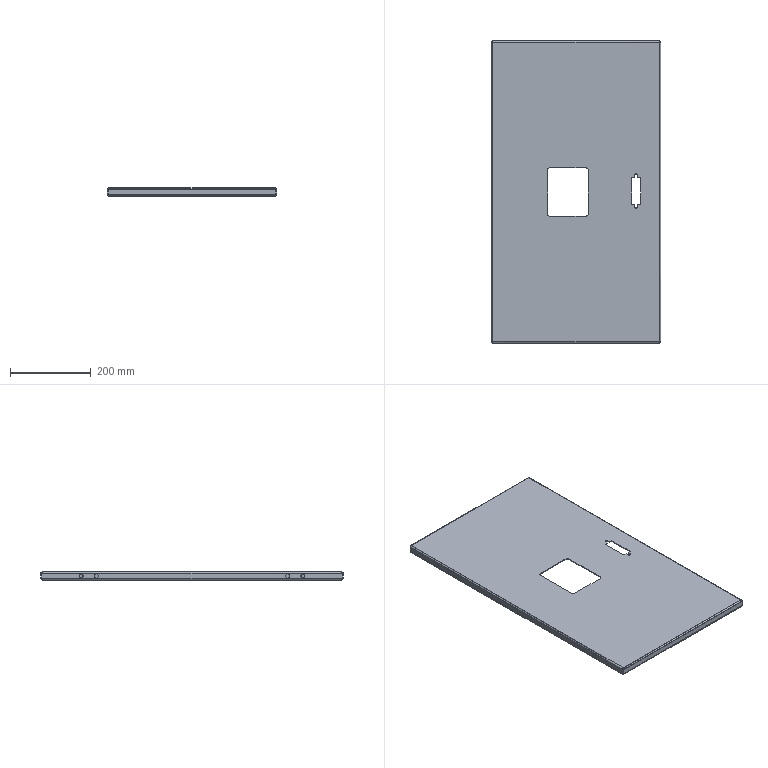Part | SolidWorks | features ICE 3, EdgeFlange 2, FlatPattern 1, SMBaseFlange 1, SheetMetal 1 | 1 solid | 106 faces | box 420 x 750 x 20 mm | volume 745969 mm3 | plane 60 | cylinder 30 | spline 16 | commonest cylinder face diameters 7 x10 4 x8 8 x8 10 x4